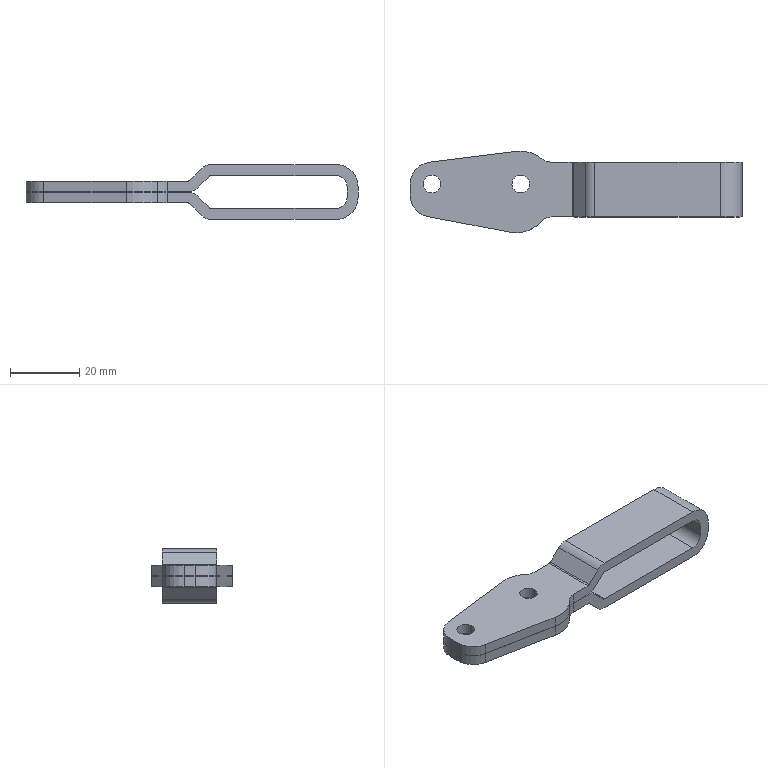Part | SolidWorks | features Fillet 9, Cut 3, Boss 1, Extrusion 1 | 1 solid | 54 faces | box 96.012 x 23.622 x 15.875 mm | volume 10658 mm3 | cylinder 32 | plane 22 | commonest cylinder face diameters 5.08 x8 7.62 x8 12.7 x6 1.27 x4 19.05 x4 6.35 x2